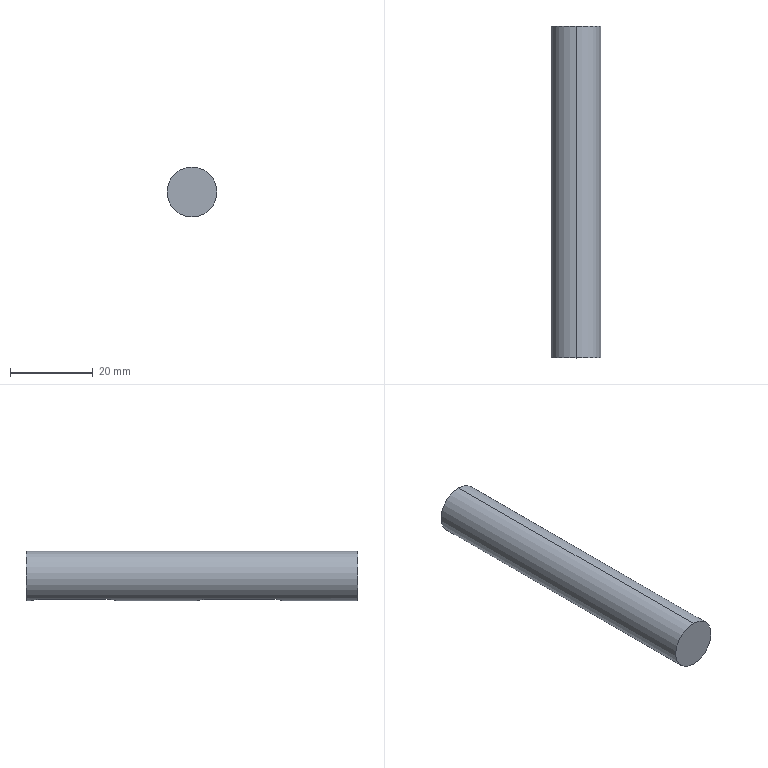Part | 1 solid | 14 faces | box 12 x 80 x 12 mm | volume 8743 mm3 | plane 8 | cylinder 6 | commonest cylinder face diameters 4 x4 12 x2
STEP:
#1=CARTESIAN_POINT('',(0.,80.,6.));
#2=VERTEX_POINT('',#1);
#3=CARTESIAN_POINT('',(0.,80.,-6.));
#4=VERTEX_POINT('',#3);
#5=CARTESIAN_POINT('',(0.,80.,0.));
#6=DIRECTION('',(0.,1.,0.));
#7=DIRECTION('',(0.,0.,1.));
#8=AXIS2_PLACEMENT_3D('',#5,#6,#7);
#9=CIRCLE('',#8,6.);
#10=EDGE_CURVE('',#2,#4,#9,.T.);
#11=ORIENTED_EDGE('',*,*,#10,.F.);
#12=CARTESIAN_POINT('',(0.,0.,6.));
#13=VERTEX_POINT('',#12);
#14=CARTESIAN_POINT('',(0.,80.,6.));
#15=DIRECTION('',(0.,-1.,0.));
#16=VECTOR('',#15,1000.);
#17=LINE('',#14,#16);
#18=EDGE_CURVE('',#2,#13,#17,.T.);
#19=ORIENTED_EDGE('',*,*,#18,.T.);
#20=CARTESIAN_POINT('',(0.,0.,-6.));
#21=VERTEX_POINT('',#20);
#22=CARTESIAN_POINT('',(0.,0.,0.));
#23=DIRECTION('',(0.,1.,0.));
#24=DIRECTION('',(0.,0.,1.));
#25=AXIS2_PLACEMENT_3D('',#22,#23,#24);
#26=CIRCLE('',#25,6.);
#27=EDGE_CURVE('',#13,#21,#26,.T.);
#28=ORIENTED_EDGE('',*,*,#27,.T.);
#29=CARTESIAN_POINT('',(0.,18.,-6.));
#30=VERTEX_POINT('',#29);
#31=CARTESIAN_POINT('',(0.,80.,-6.));
#32=DIRECTION('',(0.,-1.,0.));
#33=VECTOR('',#32,1000.);
#34=LINE('',#31,#33);
#35=EDGE_CURVE('',#30,#21,#34,.T.);
#36=ORIENTED_EDGE('',*,*,#35,.F.);
#37=CARTESIAN_POINT('',(2.,20.,-5.657));
#38=VERTEX_POINT('',#37);
#39=CARTESIAN_POINT('',(0.,18.,-6.));
#40=CARTESIAN_POINT('',(0.2623,18.,-6.));
#41=CARTESIAN_POINT('',(0.5271,18.053,-5.982));
#42=CARTESIAN_POINT('',(0.889,18.204,-5.935));
#43=CARTESIAN_POINT('',(1.006,18.267,-5.916));
#44=CARTESIAN_POINT('',(1.222,18.411,-5.875));
#45=CARTESIAN_POINT('',(1.322,18.494,-5.853));
#46=CARTESIAN_POINT('',(1.599,18.771,-5.786));
#47=CARTESIAN_POINT('',(1.745,18.989,-5.741));
#48=CARTESIAN_POINT('',(1.897,19.353,-5.692));
#49=CARTESIAN_POINT('',(1.935,19.478,-5.679));
#50=CARTESIAN_POINT('',(1.987,19.735,-5.662));
#51=CARTESIAN_POINT('',(2.,19.868,-5.657));
#52=CARTESIAN_POINT('',(2.,20.,-5.657));
#53=B_SPLINE_CURVE_WITH_KNOTS('',3,(#39,#40,#41,#42,#43,#44,#45,#46,#47,#48,#49,#50,#51,#52),.UNSPECIFIED.,.F.,.F.,(4,2,2,2,2,2,4),(0.006298,0.007085,0.007479,0.007872,0.008659,0.009053,0.009446),.UNSPECIFIED.);
#54=EDGE_CURVE('',#30,#38,#53,.T.);
#55=ORIENTED_EDGE('',*,*,#54,.T.);
#56=CARTESIAN_POINT('',(2.,37.,-5.657));
#57=VERTEX_POINT('',#56);
#58=CARTESIAN_POINT('',(2.,80.,-5.657));
#59=DIRECTION('',(0.,1.,0.));
#60=VECTOR('',#59,1000.);
#61=LINE('',#58,#60);
#62=EDGE_CURVE('',#38,#57,#61,.T.);
#63=ORIENTED_EDGE('',*,*,#62,.T.);
#64=CARTESIAN_POINT('',(0.,39.,-6.));
#65=VERTEX_POINT('',#64);
#66=CARTESIAN_POINT('',(2.,37.,-5.657));
#67=CARTESIAN_POINT('',(2.,37.132,-5.657));
#68=CARTESIAN_POINT('',(1.987,37.262,-5.661));
#69=CARTESIAN_POINT('',(1.935,37.521,-5.679));
#70=CARTESIAN_POINT('',(1.897,37.648,-5.693));
#71=CARTESIAN_POINT('',(1.746,38.009,-5.741));
#72=CARTESIAN_POINT('',(1.598,38.231,-5.786));
#73=CARTESIAN_POINT('',(1.323,38.506,-5.853));
#74=CARTESIAN_POINT('',(1.221,38.59,-5.876));
#75=CARTESIAN_POINT('',(1.005,38.734,-5.916));
#76=CARTESIAN_POINT('',(0.8903,38.796,-5.935));
#77=CARTESIAN_POINT('',(0.6484,38.896,-5.966));
#78=CARTESIAN_POINT('',(0.5209,38.935,-5.979));
#79=CARTESIAN_POINT('',(0.264,38.987,-5.996));
#80=CARTESIAN_POINT('',(0.1331,39.,-6.));
#81=CARTESIAN_POINT('',(0.,39.,-6.));
#82=B_SPLINE_CURVE_WITH_KNOTS('',3,(#66,#67,#68,#69,#70,#71,#72,#73,#74,#75,#76,#77,#78,#79,#80,#81),.UNSPECIFIED.,.F.,.F.,(4,2,2,2,2,2,2,4),(0.009446,0.00984,0.01023,0.01102,0.01141,0.01181,0.0122,0.0126),.UNSPECIFIED.);
#83=EDGE_CURVE('',#57,#65,#82,.T.);
#84=ORIENTED_EDGE('',*,*,#83,.T.);
#85=CARTESIAN_POINT('',(0.,58.,-6.));
#86=VERTEX_POINT('',#85);
#87=CARTESIAN_POINT('',(0.,80.,-6.));
#88=DIRECTION('',(0.,-1.,0.));
#89=VECTOR('',#88,1000.);
#90=LINE('',#87,#89);
#91=EDGE_CURVE('',#86,#65,#90,.T.);
#92=ORIENTED_EDGE('',*,*,#91,.F.);
#93=CARTESIAN_POINT('',(2.,60.,-5.657));
#94=VERTEX_POINT('',#93);
#95=CARTESIAN_POINT('',(0.,58.,-6.));
#96=CARTESIAN_POINT('',(0.2623,58.,-6.));
#97=CARTESIAN_POINT('',(0.5271,58.053,-5.982));
#98=CARTESIAN_POINT('',(0.889,58.204,-5.935));
#99=CARTESIAN_POINT('',(1.006,58.267,-5.916));
#100=CARTESIAN_POINT('',(1.222,58.411,-5.875));
#101=CARTESIAN_POINT('',(1.322,58.494,-5.853));
#102=CARTESIAN_POINT('',(1.599,58.771,-5.786));
#103=CARTESIAN_POINT('',(1.745,58.989,-5.741));
#104=CARTESIAN_POINT('',(1.897,59.353,-5.692));
#105=CARTESIAN_POINT('',(1.935,59.478,-5.679));
#106=CARTESIAN_POINT('',(1.987,59.735,-5.662));
#107=CARTESIAN_POINT('',(2.,59.868,-5.657));
#108=CARTESIAN_POINT('',(2.,60.,-5.657));
#109=B_SPLINE_CURVE_WITH_KNOTS('',3,(#95,#96,#97,#98,#99,#100,#101,#102,#103,#104,#105,#106,#107,#108),.UNSPECIFIED.,.F.,.F.,(4,2,2,2,2,2,4),(0.006298,0.007085,0.007479,0.007872,0.008659,0.009053,0.009446),.UNSPECIFIED.);
#110=EDGE_CURVE('',#86,#94,#109,.T.);
#111=ORIENTED_EDGE('',*,*,#110,.T.);
#112=CARTESIAN_POINT('',(2.,77.,-5.657));
#113=VERTEX_POINT('',#112);
#114=CARTESIAN_POINT('',(2.,80.,-5.657));
#115=DIRECTION('',(0.,1.,0.));
#116=VECTOR('',#115,1000.);
#117=LINE('',#114,#116);
#118=EDGE_CURVE('',#94,#113,#117,.T.);
#119=ORIENTED_EDGE('',*,*,#118,.T.);
#120=CARTESIAN_POINT('',(0.,79.,-6.));
#121=VERTEX_POINT('',#120);
#122=CARTESIAN_POINT('',(2.,77.,-5.657));
#123=CARTESIAN_POINT('',(2.,77.132,-5.657));
#124=CARTESIAN_POINT('',(1.987,77.262,-5.661));
#125=CARTESIAN_POINT('',(1.935,77.521,-5.679));
#126=CARTESIAN_POINT('',(1.897,77.648,-5.693));
#127=CARTESIAN_POINT('',(1.746,78.009,-5.741));
#128=CARTESIAN_POINT('',(1.598,78.231,-5.786));
#129=CARTESIAN_POINT('',(1.323,78.506,-5.853));
#130=CARTESIAN_POINT('',(1.221,78.59,-5.876));
#131=CARTESIAN_POINT('',(1.005,78.734,-5.916));
#132=CARTESIAN_POINT('',(0.8903,78.796,-5.935));
#133=CARTESIAN_POINT('',(0.6484,78.896,-5.966));
#134=CARTESIAN_POINT('',(0.5209,78.935,-5.979));
#135=CARTESIAN_POINT('',(0.264,78.987,-5.996));
#136=CARTESIAN_POINT('',(0.1331,79.,-6.));
#137=CARTESIAN_POINT('',(0.,79.,-6.));
#138=B_SPLINE_CURVE_WITH_KNOTS('',3,(#122,#123,#124,#125,#126,#127,#128,#129,#130,#131,#132,#133,#134,#135,#136,#137),.UNSPECIFIED.,.F.,.F.,(4,2,2,2,2,2,2,4),(0.009446,0.00984,0.01023,0.01102,0.01141,0.01181,0.0122,0.0126),.UNSPECIFIED.);
#139=EDGE_CURVE('',#113,#121,#138,.T.);
#140=ORIENTED_EDGE('',*,*,#139,.T.);
#141=CARTESIAN_POINT('',(0.,80.,-6.));
#142=DIRECTION('',(0.,-1.,0.));
#143=VECTOR('',#142,1000.);
#144=LINE('',#141,#143);
#145=EDGE_CURVE('',#4,#121,#144,.T.);
#146=ORIENTED_EDGE('',*,*,#145,.F.);
#147=EDGE_LOOP('',(#11,#19,#28,#36,#55,#63,#84,#92,#111,#119,#140,#146));
#148=FACE_OUTER_BOUND('',#147,.T.);
#149=CARTESIAN_POINT('',(0.,80.,0.));
#150=DIRECTION('',(0.,-1.,0.));
#151=DIRECTION('',(0.,0.,-1.));
#152=AXIS2_PLACEMENT_3D('',#149,#150,#151);
#153=CYLINDRICAL_SURFACE('',#152,6.);
#154=ADVANCED_FACE('',(#148),#153,.T.);
#155=ORIENTED_EDGE('',*,*,#18,.F.);
#156=CARTESIAN_POINT('',(0.,80.,0.));
#157=DIRECTION('',(0.,1.,0.));
#158=DIRECTION('',(0.,0.,1.));
#159=AXIS2_PLACEMENT_3D('',#156,#157,#158);
#160=CIRCLE('',#159,6.);
#161=EDGE_CURVE('',#4,#2,#160,.T.);
#162=ORIENTED_EDGE('',*,*,#161,.F.);
#163=ORIENTED_EDGE('',*,*,#145,.T.);
#164=CARTESIAN_POINT('',(-2.,77.,-5.657));
#165=VERTEX_POINT('',#164);
#166=CARTESIAN_POINT('',(0.,79.,-6.));
#167=CARTESIAN_POINT('',(-0.1332,79.,-6.));
#168=CARTESIAN_POINT('',(-0.264,78.987,-5.996));
#169=CARTESIAN_POINT('',(-0.5211,78.935,-5.979));
#170=CARTESIAN_POINT('',(-0.6487,78.896,-5.966));
#171=CARTESIAN_POINT('',(-0.8906,78.796,-5.935));
#172=CARTESIAN_POINT('',(-1.005,78.734,-5.916));
#173=CARTESIAN_POINT('',(-1.222,78.589,-5.875));
#174=CARTESIAN_POINT('',(-1.324,78.505,-5.853));
#175=CARTESIAN_POINT('',(-1.598,78.23,-5.786));
#176=CARTESIAN_POINT('',(-1.747,78.008,-5.741));
#177=CARTESIAN_POINT('',(-1.897,77.648,-5.693));
#178=CARTESIAN_POINT('',(-1.936,77.521,-5.679));
#179=CARTESIAN_POINT('',(-1.987,77.262,-5.661));
#180=CARTESIAN_POINT('',(-2.,77.132,-5.657));
#181=CARTESIAN_POINT('',(-2.,77.,-5.657));
#182=B_SPLINE_CURVE_WITH_KNOTS('',3,(#166,#167,#168,#169,#170,#171,#172,#173,#174,#175,#176,#177,#178,#179,#180,#181),.UNSPECIFIED.,.F.,.F.,(4,2,2,2,2,2,2,4),(0.,0.0003938,0.0007875,0.001181,0.001575,0.002363,0.002756,0.00315),.UNSPECIFIED.);
#183=EDGE_CURVE('',#121,#165,#182,.T.);
#184=ORIENTED_EDGE('',*,*,#183,.T.);
#185=CARTESIAN_POINT('',(-2.,60.,-5.657));
#186=VERTEX_POINT('',#185);
#187=CARTESIAN_POINT('',(-2.,80.,-5.657));
#188=DIRECTION('',(0.,-1.,0.));
#189=VECTOR('',#188,1000.);
#190=LINE('',#187,#189);
#191=EDGE_CURVE('',#165,#186,#190,.T.);
#192=ORIENTED_EDGE('',*,*,#191,.T.);
#193=CARTESIAN_POINT('',(-2.,60.,-5.657));
#194=CARTESIAN_POINT('',(-2.,59.869,-5.657));
#195=CARTESIAN_POINT('',(-1.987,59.735,-5.662));
#196=CARTESIAN_POINT('',(-1.935,59.478,-5.679));
#197=CARTESIAN_POINT('',(-1.897,59.353,-5.693));
#198=CARTESIAN_POINT('',(-1.796,59.109,-5.725));
#199=CARTESIAN_POINT('',(-1.734,58.994,-5.745));
#200=CARTESIAN_POINT('',(-1.589,58.779,-5.786));
#201=CARTESIAN_POINT('',(-1.505,58.677,-5.809));
#202=CARTESIAN_POINT('',(-1.321,58.493,-5.853));
#203=CARTESIAN_POINT('',(-1.221,58.411,-5.875));
#204=CARTESIAN_POINT('',(-1.005,58.266,-5.916));
#205=CARTESIAN_POINT('',(-0.8882,58.203,-5.935));
#206=CARTESIAN_POINT('',(-0.6474,58.103,-5.966));
#207=CARTESIAN_POINT('',(-0.5226,58.065,-5.979));
#208=CARTESIAN_POINT('',(-0.2637,58.013,-5.996));
#209=CARTESIAN_POINT('',(-0.1311,58.,-6.));
#210=CARTESIAN_POINT('',(0.,58.,-6.));
#211=B_SPLINE_CURVE_WITH_KNOTS('',3,(#193,#194,#195,#196,#197,#198,#199,#200,#201,#202,#203,#204,#205,#206,#207,#208,#209,#210),.UNSPECIFIED.,.F.,.F.,(4,2,2,2,2,2,2,2,4),(0.00315,0.003544,0.003937,0.004331,0.004724,0.005118,0.005511,0.005905,0.006298),.UNSPECIFIED.);
#212=EDGE_CURVE('',#186,#86,#211,.T.);
#213=ORIENTED_EDGE('',*,*,#212,.T.);
#214=ORIENTED_EDGE('',*,*,#91,.T.);
#215=CARTESIAN_POINT('',(-2.,37.,-5.657));
#216=VERTEX_POINT('',#215);
#217=CARTESIAN_POINT('',(0.,39.,-6.));
#218=CARTESIAN_POINT('',(-0.1332,39.,-6.));
#219=CARTESIAN_POINT('',(-0.264,38.987,-5.996));
#220=CARTESIAN_POINT('',(-0.5211,38.935,-5.979));
#221=CARTESIAN_POINT('',(-0.6487,38.896,-5.966));
#222=CARTESIAN_POINT('',(-0.8906,38.796,-5.935));
#223=CARTESIAN_POINT('',(-1.005,38.734,-5.916));
#224=CARTESIAN_POINT('',(-1.222,38.589,-5.875));
#225=CARTESIAN_POINT('',(-1.324,38.505,-5.853));
#226=CARTESIAN_POINT('',(-1.598,38.23,-5.786));
#227=CARTESIAN_POINT('',(-1.747,38.008,-5.741));
#228=CARTESIAN_POINT('',(-1.897,37.648,-5.693));
#229=CARTESIAN_POINT('',(-1.936,37.521,-5.679));
#230=CARTESIAN_POINT('',(-1.987,37.262,-5.661));
#231=CARTESIAN_POINT('',(-2.,37.132,-5.657));
#232=CARTESIAN_POINT('',(-2.,37.,-5.657));
#233=B_SPLINE_CURVE_WITH_KNOTS('',3,(#217,#218,#219,#220,#221,#222,#223,#224,#225,#226,#227,#228,#229,#230,#231,#232),.UNSPECIFIED.,.F.,.F.,(4,2,2,2,2,2,2,4),(0.,0.0003938,0.0007875,0.001181,0.001575,0.002363,0.002756,0.00315),.UNSPECIFIED.);
#234=EDGE_CURVE('',#65,#216,#233,.T.);
#235=ORIENTED_EDGE('',*,*,#234,.T.);
#236=CARTESIAN_POINT('',(-2.,20.,-5.657));
#237=VERTEX_POINT('',#236);
#238=CARTESIAN_POINT('',(-2.,80.,-5.657));
#239=DIRECTION('',(0.,-1.,0.));
#240=VECTOR('',#239,1000.);
#241=LINE('',#238,#240);
#242=EDGE_CURVE('',#216,#237,#241,.T.);
#243=ORIENTED_EDGE('',*,*,#242,.T.);
#244=CARTESIAN_POINT('',(-2.,20.,-5.657));
#245=CARTESIAN_POINT('',(-2.,19.869,-5.657));
#246=CARTESIAN_POINT('',(-1.987,19.735,-5.662));
#247=CARTESIAN_POINT('',(-1.935,19.478,-5.679));
#248=CARTESIAN_POINT('',(-1.897,19.353,-5.693));
#249=CARTESIAN_POINT('',(-1.796,19.109,-5.725));
#250=CARTESIAN_POINT('',(-1.734,18.994,-5.745));
#251=CARTESIAN_POINT('',(-1.589,18.779,-5.786));
#252=CARTESIAN_POINT('',(-1.505,18.677,-5.809));
#253=CARTESIAN_POINT('',(-1.321,18.493,-5.853));
#254=CARTESIAN_POINT('',(-1.221,18.411,-5.875));
#255=CARTESIAN_POINT('',(-1.005,18.266,-5.916));
#256=CARTESIAN_POINT('',(-0.8882,18.203,-5.935));
#257=CARTESIAN_POINT('',(-0.6474,18.103,-5.966));
#258=CARTESIAN_POINT('',(-0.5226,18.065,-5.979));
#259=CARTESIAN_POINT('',(-0.2637,18.013,-5.996));
#260=CARTESIAN_POINT('',(-0.1311,18.,-6.));
#261=CARTESIAN_POINT('',(0.,18.,-6.));
#262=B_SPLINE_CURVE_WITH_KNOTS('',3,(#244,#245,#246,#247,#248,#249,#250,#251,#252,#253,#254,#255,#256,#257,#258,#259,#260,#261),.UNSPECIFIED.,.F.,.F.,(4,2,2,2,2,2,2,2,4),(0.00315,0.003544,0.003937,0.004331,0.004724,0.005118,0.005511,0.005905,0.006298),.UNSPECIFIED.);
#263=EDGE_CURVE('',#237,#30,#262,.T.);
#264=ORIENTED_EDGE('',*,*,#263,.T.);
#265=ORIENTED_EDGE('',*,*,#35,.T.);
#266=CARTESIAN_POINT('',(0.,0.,0.));
#267=DIRECTION('',(0.,1.,0.));
#268=DIRECTION('',(0.,0.,1.));
#269=AXIS2_PLACEMENT_3D('',#266,#267,#268);
#270=CIRCLE('',#269,6.);
#271=EDGE_CURVE('',#21,#13,#270,.T.);
#272=ORIENTED_EDGE('',*,*,#271,.T.);
#273=EDGE_LOOP('',(#155,#162,#163,#184,#192,#213,#214,#235,#243,#264,#265,#272));
#274=FACE_OUTER_BOUND('',#273,.T.);
#275=CARTESIAN_POINT('',(0.,80.,0.));
#276=DIRECTION('',(0.,-1.,0.));
#277=DIRECTION('',(0.,0.,-1.));
#278=AXIS2_PLACEMENT_3D('',#275,#276,#277);
#279=CYLINDRICAL_SURFACE('',#278,6.);
#280=ADVANCED_FACE('',(#274),#279,.T.);
#281=ORIENTED_EDGE('',*,*,#161,.T.);
#282=ORIENTED_EDGE('',*,*,#10,.T.);
#283=EDGE_LOOP('',(#281,#282));
#284=FACE_OUTER_BOUND('',#283,.T.);
#285=CARTESIAN_POINT('',(0.,80.,0.));
#286=DIRECTION('',(0.,1.,0.));
#287=DIRECTION('',(0.,0.,1.));
#288=AXIS2_PLACEMENT_3D('',#285,#286,#287);
#289=PLANE('',#288);
#290=ADVANCED_FACE('',(#284),#289,.T.);
#291=ORIENTED_EDGE('',*,*,#271,.F.);
#292=ORIENTED_EDGE('',*,*,#27,.F.);
#293=EDGE_LOOP('',(#291,#292));
#294=FACE_OUTER_BOUND('',#293,.T.);
#295=CARTESIAN_POINT('',(0.,0.,0.));
#296=DIRECTION('',(0.,1.,0.));
#297=DIRECTION('',(0.,0.,1.));
#298=AXIS2_PLACEMENT_3D('',#295,#296,#297);
#299=PLANE('',#298);
#300=ADVANCED_FACE('',(#294),#299,.F.);
#301=CARTESIAN_POINT('',(2.,37.,-4.));
#302=VERTEX_POINT('',#301);
#303=CARTESIAN_POINT('',(2.,37.,-84.));
#304=DIRECTION('',(0.,0.,1.));
#305=VECTOR('',#304,1000.);
#306=LINE('',#303,#305);
#307=EDGE_CURVE('',#57,#302,#306,.T.);
#308=ORIENTED_EDGE('',*,*,#307,.T.);
#309=CARTESIAN_POINT('',(-2.,37.,-4.));
#310=VERTEX_POINT('',#309);
#311=CARTESIAN_POINT('',(0.,37.,-4.));
#312=DIRECTION('',(0.,0.,1.));
#313=DIRECTION('',(1.,0.,0.));
#314=AXIS2_PLACEMENT_3D('',#311,#312,#313);
#315=CIRCLE('',#314,2.);
#316=EDGE_CURVE('',#302,#310,#315,.T.);
#317=ORIENTED_EDGE('',*,*,#316,.T.);
#318=CARTESIAN_POINT('',(-2.,37.,-84.));
#319=DIRECTION('',(0.,0.,1.));
#320=VECTOR('',#319,1000.);
#321=LINE('',#318,#320);
#322=EDGE_CURVE('',#216,#310,#321,.T.);
#323=ORIENTED_EDGE('',*,*,#322,.F.);
#324=ORIENTED_EDGE('',*,*,#234,.F.);
#325=ORIENTED_EDGE('',*,*,#83,.F.);
#326=EDGE_LOOP('',(#308,#317,#323,#324,#325));
#327=FACE_OUTER_BOUND('',#326,.T.);
#328=CARTESIAN_POINT('',(0.,37.,-84.));
#329=DIRECTION('',(0.,0.,1.));
#330=DIRECTION('',(1.,0.,0.));
#331=AXIS2_PLACEMENT_3D('',#328,#329,#330);
#332=CYLINDRICAL_SURFACE('',#331,2.);
#333=ADVANCED_FACE('',(#327),#332,.F.);
#334=CARTESIAN_POINT('',(2.,20.,-4.));
#335=VERTEX_POINT('',#334);
#336=CARTESIAN_POINT('',(2.,20.,-84.));
#337=DIRECTION('',(0.,0.,1.));
#338=VECTOR('',#337,1000.);
#339=LINE('',#336,#338);
#340=EDGE_CURVE('',#38,#335,#339,.T.);
#341=ORIENTED_EDGE('',*,*,#340,.T.);
#342=CARTESIAN_POINT('',(2.,37.,-4.));
#343=DIRECTION('',(0.,1.,0.));
#344=VECTOR('',#343,1000.);
#345=LINE('',#342,#344);
#346=EDGE_CURVE('',#335,#302,#345,.T.);
#347=ORIENTED_EDGE('',*,*,#346,.T.);
#348=ORIENTED_EDGE('',*,*,#307,.F.);
#349=ORIENTED_EDGE('',*,*,#62,.F.);
#350=EDGE_LOOP('',(#341,#347,#348,#349));
#351=FACE_OUTER_BOUND('',#350,.T.);
#352=CARTESIAN_POINT('',(2.,37.,-84.));
#353=DIRECTION('',(1.,0.,0.));
#354=DIRECTION('',(0.,1.,0.));
#355=AXIS2_PLACEMENT_3D('',#352,#353,#354);
#356=PLANE('',#355);
#357=ADVANCED_FACE('',(#351),#356,.F.);
#358=CARTESIAN_POINT('',(-2.,20.,-4.));
#359=VERTEX_POINT('',#358);
#360=CARTESIAN_POINT('',(-2.,20.,-84.));
#361=DIRECTION('',(0.,0.,1.));
#362=VECTOR('',#361,1000.);
#363=LINE('',#360,#362);
#364=EDGE_CURVE('',#237,#359,#363,.T.);
#365=ORIENTED_EDGE('',*,*,#364,.T.);
#366=CARTESIAN_POINT('',(0.,20.,-4.));
#367=DIRECTION('',(0.,0.,1.));
#368=DIRECTION('',(1.,0.,0.));
#369=AXIS2_PLACEMENT_3D('',#366,#367,#368);
#370=CIRCLE('',#369,2.);
#371=EDGE_CURVE('',#359,#335,#370,.T.);
#372=ORIENTED_EDGE('',*,*,#371,.T.);
#373=ORIENTED_EDGE('',*,*,#340,.F.);
#374=ORIENTED_EDGE('',*,*,#54,.F.);
#375=ORIENTED_EDGE('',*,*,#263,.F.);
#376=EDGE_LOOP('',(#365,#372,#373,#374,#375));
#377=FACE_OUTER_BOUND('',#376,.T.);
#378=CARTESIAN_POINT('',(0.,20.,-84.));
#379=DIRECTION('',(0.,0.,1.));
#380=DIRECTION('',(1.,0.,0.));
#381=AXIS2_PLACEMENT_3D('',#378,#379,#380);
#382=CYLINDRICAL_SURFACE('',#381,2.);
#383=ADVANCED_FACE('',(#377),#382,.F.);
#384=ORIENTED_EDGE('',*,*,#322,.T.);
#385=CARTESIAN_POINT('',(-2.,37.,-4.));
#386=DIRECTION('',(0.,-1.,0.));
#387=VECTOR('',#386,1000.);
#388=LINE('',#385,#387);
#389=EDGE_CURVE('',#310,#359,#388,.T.);
#390=ORIENTED_EDGE('',*,*,#389,.T.);
#391=ORIENTED_EDGE('',*,*,#364,.F.);
#392=ORIENTED_EDGE('',*,*,#242,.F.);
#393=EDGE_LOOP('',(#384,#390,#391,#392));
#394=FACE_OUTER_BOUND('',#393,.T.);
#395=CARTESIAN_POINT('',(-2.,37.,-84.));
#396=DIRECTION('',(-1.,0.,0.));
#397=DIRECTION('',(0.,-1.,0.));
#398=AXIS2_PLACEMENT_3D('',#395,#396,#397);
#399=PLANE('',#398);
#400=ADVANCED_FACE('',(#394),#399,.F.);
#401=ORIENTED_EDGE('',*,*,#316,.F.);
#402=ORIENTED_EDGE('',*,*,#346,.F.);
#403=ORIENTED_EDGE('',*,*,#371,.F.);
#404=ORIENTED_EDGE('',*,*,#389,.F.);
#405=EDGE_LOOP('',(#401,#402,#403,#404));
#406=FACE_OUTER_BOUND('',#405,.T.);
#407=CARTESIAN_POINT('',(0.,37.,-4.));
#408=DIRECTION('',(0.,0.,1.));
#409=DIRECTION('',(1.,0.,0.));
#410=AXIS2_PLACEMENT_3D('',#407,#408,#409);
#411=PLANE('',#410);
#412=ADVANCED_FACE('',(#406),#411,.F.);
#413=CARTESIAN_POINT('',(-2.,60.,-4.));
#414=VERTEX_POINT('',#413);
#415=CARTESIAN_POINT('',(-2.,60.,-84.));
#416=DIRECTION('',(0.,0.,1.));
#417=VECTOR('',#416,1000.);
#418=LINE('',#415,#417);
#419=EDGE_CURVE('',#186,#414,#418,.T.);
#420=ORIENTED_EDGE('',*,*,#419,.T.);
#421=CARTESIAN_POINT('',(2.,60.,-4.));
#422=VERTEX_POINT('',#421);
#423=CARTESIAN_POINT('',(0.,60.,-4.));
#424=DIRECTION('',(0.,0.,1.));
#425=DIRECTION('',(1.,0.,0.));
#426=AXIS2_PLACEMENT_3D('',#423,#424,#425);
#427=CIRCLE('',#426,2.);
#428=EDGE_CURVE('',#414,#422,#427,.T.);
#429=ORIENTED_EDGE('',*,*,#428,.T.);
#430=CARTESIAN_POINT('',(2.,60.,-84.));
#431=DIRECTION('',(0.,0.,1.));
#432=VECTOR('',#431,1000.);
#433=LINE('',#430,#432);
#434=EDGE_CURVE('',#94,#422,#433,.T.);
#435=ORIENTED_EDGE('',*,*,#434,.F.);
#436=ORIENTED_EDGE('',*,*,#110,.F.);
#437=ORIENTED_EDGE('',*,*,#212,.F.);
#438=EDGE_LOOP('',(#420,#429,#435,#436,#437));
#439=FACE_OUTER_BOUND('',#438,.T.);
#440=CARTESIAN_POINT('',(0.,60.,-84.));
#441=DIRECTION('',(0.,0.,1.));
#442=DIRECTION('',(1.,0.,0.));
#443=AXIS2_PLACEMENT_3D('',#440,#441,#442);
#444=CYLINDRICAL_SURFACE('',#443,2.);
#445=ADVANCED_FACE('',(#439),#444,.F.);
#446=CARTESIAN_POINT('',(-2.,77.,-4.));
#447=VERTEX_POINT('',#446);
#448=CARTESIAN_POINT('',(-2.,77.,-84.));
#449=DIRECTION('',(0.,0.,1.));
#450=VECTOR('',#449,1000.);
#451=LINE('',#448,#450);
#452=EDGE_CURVE('',#165,#447,#451,.T.);
#453=ORIENTED_EDGE('',*,*,#452,.T.);
#454=CARTESIAN_POINT('',(-2.,60.,-4.));
#455=DIRECTION('',(0.,-1.,0.));
#456=VECTOR('',#455,1000.);
#457=LINE('',#454,#456);
#458=EDGE_CURVE('',#447,#414,#457,.T.);
#459=ORIENTED_EDGE('',*,*,#458,.T.);
#460=ORIENTED_EDGE('',*,*,#419,.F.);
#461=ORIENTED_EDGE('',*,*,#191,.F.);
#462=EDGE_LOOP('',(#453,#459,#460,#461));
#463=FACE_OUTER_BOUND('',#462,.T.);
#464=CARTESIAN_POINT('',(-2.,60.,-84.));
#465=DIRECTION('',(-1.,0.,0.));
#466=DIRECTION('',(0.,0.,1.));
#467=AXIS2_PLACEMENT_3D('',#464,#465,#466);
#468=PLANE('',#467);
#469=ADVANCED_FACE('',(#463),#468,.F.);
#470=CARTESIAN_POINT('',(2.,77.,-4.));
#471=VERTEX_POINT('',#470);
#472=CARTESIAN_POINT('',(2.,77.,-84.));
#473=DIRECTION('',(0.,0.,1.));
#474=VECTOR('',#473,1000.);
#475=LINE('',#472,#474);
#476=EDGE_CURVE('',#113,#471,#475,.T.);
#477=ORIENTED_EDGE('',*,*,#476,.T.);
#478=CARTESIAN_POINT('',(0.,77.,-4.));
#479=DIRECTION('',(0.,0.,1.));
#480=DIRECTION('',(1.,0.,0.));
#481=AXIS2_PLACEMENT_3D('',#478,#479,#480);
#482=CIRCLE('',#481,2.);
#483=EDGE_CURVE('',#471,#447,#482,.T.);
#484=ORIENTED_EDGE('',*,*,#483,.T.);
#485=ORIENTED_EDGE('',*,*,#452,.F.);
#486=ORIENTED_EDGE('',*,*,#183,.F.);
#487=ORIENTED_EDGE('',*,*,#139,.F.);
#488=EDGE_LOOP('',(#477,#484,#485,#486,#487));
#489=FACE_OUTER_BOUND('',#488,.T.);
#490=CARTESIAN_POINT('',(0.,77.,-84.));
#491=DIRECTION('',(0.,0.,1.));
#492=DIRECTION('',(1.,0.,0.));
#493=AXIS2_PLACEMENT_3D('',#490,#491,#492);
#494=CYLINDRICAL_SURFACE('',#493,2.);
#495=ADVANCED_FACE('',(#489),#494,.F.);
#496=ORIENTED_EDGE('',*,*,#434,.T.);
#497=CARTESIAN_POINT('',(2.,60.,-4.));
#498=DIRECTION('',(0.,1.,0.));
#499=VECTOR('',#498,1000.);
#500=LINE('',#497,#499);
#501=EDGE_CURVE('',#422,#471,#500,.T.);
#502=ORIENTED_EDGE('',*,*,#501,.T.);
#503=ORIENTED_EDGE('',*,*,#476,.F.);
#504=ORIENTED_EDGE('',*,*,#118,.F.);
#505=EDGE_LOOP('',(#496,#502,#503,#504));
#506=FACE_OUTER_BOUND('',#505,.T.);
#507=CARTESIAN_POINT('',(2.,60.,-84.));
#508=DIRECTION('',(1.,0.,0.));
#509=DIRECTION('',(0.,0.,-1.));
#510=AXIS2_PLACEMENT_3D('',#507,#508,#509);
#511=PLANE('',#510);
#512=ADVANCED_FACE('',(#506),#511,.F.);
#513=ORIENTED_EDGE('',*,*,#428,.F.);
#514=ORIENTED_EDGE('',*,*,#458,.F.);
#515=ORIENTED_EDGE('',*,*,#483,.F.);
#516=ORIENTED_EDGE('',*,*,#501,.F.);
#517=EDGE_LOOP('',(#513,#514,#515,#516));
#518=FACE_OUTER_BOUND('',#517,.T.);
#519=CARTESIAN_POINT('',(0.,60.,-4.));
#520=DIRECTION('',(0.,0.,1.));
#521=DIRECTION('',(1.,0.,0.));
#522=AXIS2_PLACEMENT_3D('',#519,#520,#521);
#523=PLANE('',#522);
#524=ADVANCED_FACE('',(#518),#523,.F.);
#525=CLOSED_SHELL('',(#154,#280,#290,#300,#333,#357,#383,#400,#412,#445,#469,#495,#512,#524));
#526=MANIFOLD_SOLID_BREP('',#525);
#527=CARTESIAN_POINT('',(0.,0.,0.));
#528=DIRECTION('',(0.,0.,1.));
#529=DIRECTION('',(1.,0.,0.));
#530=AXIS2_PLACEMENT_3D('',#527,#528,#529);
#531=(LENGTH_UNIT()NAMED_UNIT(*)SI_UNIT(.MILLI.,.METRE.));
#532=UNCERTAINTY_MEASURE_WITH_UNIT(LENGTH_MEASURE(0.00001),#531,'','');
#533=(NAMED_UNIT(*)PLANE_ANGLE_UNIT()SI_UNIT($,.RADIAN.));
#534=(NAMED_UNIT(*)SI_UNIT($,.STERADIAN.)SOLID_ANGLE_UNIT());
#535=(GEOMETRIC_REPRESENTATION_CONTEXT(3)GLOBAL_UNCERTAINTY_ASSIGNED_CONTEXT((#532))GLOBAL_UNIT_ASSIGNED_CONTEXT((#531,#533,#534))REPRESENTATION_CONTEXT('',''));
#536=ADVANCED_BREP_SHAPE_REPRESENTATION('',(#526,#530),#535);